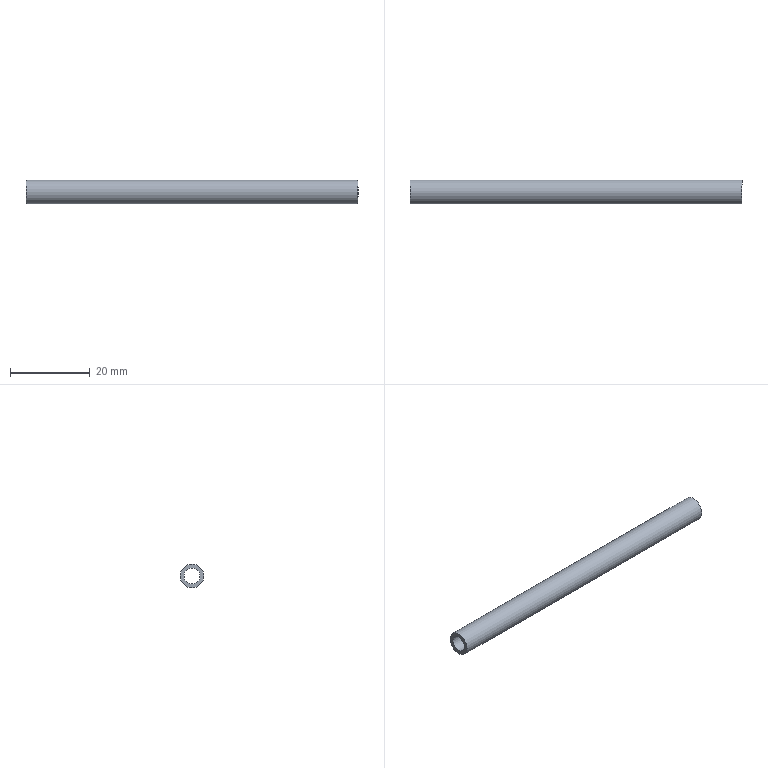Part | NX | features solid 2 | 1 solid | 4 faces | box 83.315 x 6 x 6 mm | volume 1309 mm3 | cylinder 2 | plane 2 | commonest cylinder face diameters 4 x1 6 x1
STEP:
#1=CARTESIAN_POINT('',(-153.315,53.,347.));
#2=VERTEX_POINT('',#1);
#3=CARTESIAN_POINT('',(-153.315,51.,347.));
#4=DIRECTION('',(1.,0.,0.));
#5=DIRECTION('',(0.,1.,0.));
#6=AXIS2_PLACEMENT_3D('',#3,#4,#5);
#7=CIRCLE('',#6,2.);
#8=EDGE_CURVE('',#2,#2,#7,.F.);
#9=ORIENTED_EDGE('',*,*,#8,.T.);
#10=EDGE_LOOP('',(#9));
#11=FACE_BOUND('',#10,.T.);
#12=CARTESIAN_POINT('',(-70.,49.,347.));
#13=VERTEX_POINT('',#12);
#14=CARTESIAN_POINT('',(-70.,51.,347.));
#15=DIRECTION('',(-1.,0.,0.));
#16=DIRECTION('',(0.,-1.,0.));
#17=AXIS2_PLACEMENT_3D('',#14,#15,#16);
#18=CIRCLE('',#17,2.);
#19=EDGE_CURVE('',#13,#13,#18,.T.);
#20=ORIENTED_EDGE('',*,*,#19,.F.);
#21=EDGE_LOOP('',(#20));
#22=FACE_BOUND('',#21,.T.);
#23=CARTESIAN_POINT('',(-288.824,51.,347.));
#24=DIRECTION('',(1.,0.,0.));
#25=DIRECTION('',(0.,1.,0.));
#26=AXIS2_PLACEMENT_3D('',#23,#24,#25);
#27=CYLINDRICAL_SURFACE('',#26,2.);
#28=ADVANCED_FACE('',(#11,#22),#27,.F.);
#29=CARTESIAN_POINT('',(-153.315,54.,347.));
#30=VERTEX_POINT('',#29);
#31=CARTESIAN_POINT('',(-153.315,51.,347.));
#32=DIRECTION('',(1.,0.,0.));
#33=DIRECTION('',(0.,1.,0.));
#34=AXIS2_PLACEMENT_3D('',#31,#32,#33);
#35=CIRCLE('',#34,3.);
#36=EDGE_CURVE('',#30,#30,#35,.F.);
#37=ORIENTED_EDGE('',*,*,#36,.F.);
#38=EDGE_LOOP('',(#37));
#39=FACE_BOUND('',#38,.T.);
#40=CARTESIAN_POINT('',(-70.,48.,347.));
#41=VERTEX_POINT('',#40);
#42=CARTESIAN_POINT('',(-70.,51.,347.));
#43=DIRECTION('',(-1.,0.,0.));
#44=DIRECTION('',(0.,-1.,0.));
#45=AXIS2_PLACEMENT_3D('',#42,#43,#44);
#46=CIRCLE('',#45,3.);
#47=EDGE_CURVE('',#41,#41,#46,.T.);
#48=ORIENTED_EDGE('',*,*,#47,.T.);
#49=EDGE_LOOP('',(#48));
#50=FACE_BOUND('',#49,.T.);
#51=CARTESIAN_POINT('',(-288.824,51.,347.));
#52=DIRECTION('',(1.,0.,0.));
#53=DIRECTION('',(0.,1.,0.));
#54=AXIS2_PLACEMENT_3D('',#51,#52,#53);
#55=CYLINDRICAL_SURFACE('',#54,3.);
#56=ADVANCED_FACE('',(#39,#50),#55,.T.);
#57=ORIENTED_EDGE('',*,*,#8,.F.);
#58=EDGE_LOOP('',(#57));
#59=FACE_BOUND('',#58,.T.);
#60=ORIENTED_EDGE('',*,*,#36,.T.);
#61=EDGE_LOOP('',(#60));
#62=FACE_BOUND('',#61,.T.);
#63=CARTESIAN_POINT('',(-153.315,28.272,168.));
#64=DIRECTION('',(1.,0.,0.));
#65=DIRECTION('',(0.,1.,0.));
#66=AXIS2_PLACEMENT_3D('',#63,#64,#65);
#67=PLANE('',#66);
#68=ADVANCED_FACE('',(#59,#62),#67,.F.);
#69=ORIENTED_EDGE('',*,*,#19,.T.);
#70=EDGE_LOOP('',(#69));
#71=FACE_BOUND('',#70,.T.);
#72=ORIENTED_EDGE('',*,*,#47,.F.);
#73=EDGE_LOOP('',(#72));
#74=FACE_BOUND('',#73,.T.);
#75=CARTESIAN_POINT('',(-70.,51.,347.));
#76=DIRECTION('',(-1.,0.,0.));
#77=DIRECTION('',(0.,-1.,0.));
#78=AXIS2_PLACEMENT_3D('',#75,#76,#77);
#79=PLANE('',#78);
#80=ADVANCED_FACE('',(#71,#74),#79,.F.);
#81=CLOSED_SHELL('',(#28,#56,#68,#80));
#82=MANIFOLD_SOLID_BREP('',#81);
#83=(LENGTH_UNIT()NAMED_UNIT(*)SI_UNIT(.MILLI.,.METRE.));
#84=UNCERTAINTY_MEASURE_WITH_UNIT(LENGTH_MEASURE(0.00001),#83,'','');
#85=(NAMED_UNIT(*)PLANE_ANGLE_UNIT()SI_UNIT($,.RADIAN.));
#86=(NAMED_UNIT(*)SI_UNIT($,.STERADIAN.)SOLID_ANGLE_UNIT());
#87=(GEOMETRIC_REPRESENTATION_CONTEXT(3)GLOBAL_UNCERTAINTY_ASSIGNED_CONTEXT((#84))GLOBAL_UNIT_ASSIGNED_CONTEXT((#83,#85,#86))REPRESENTATION_CONTEXT('',''));
#88=ADVANCED_BREP_SHAPE_REPRESENTATION('',(#82),#87);